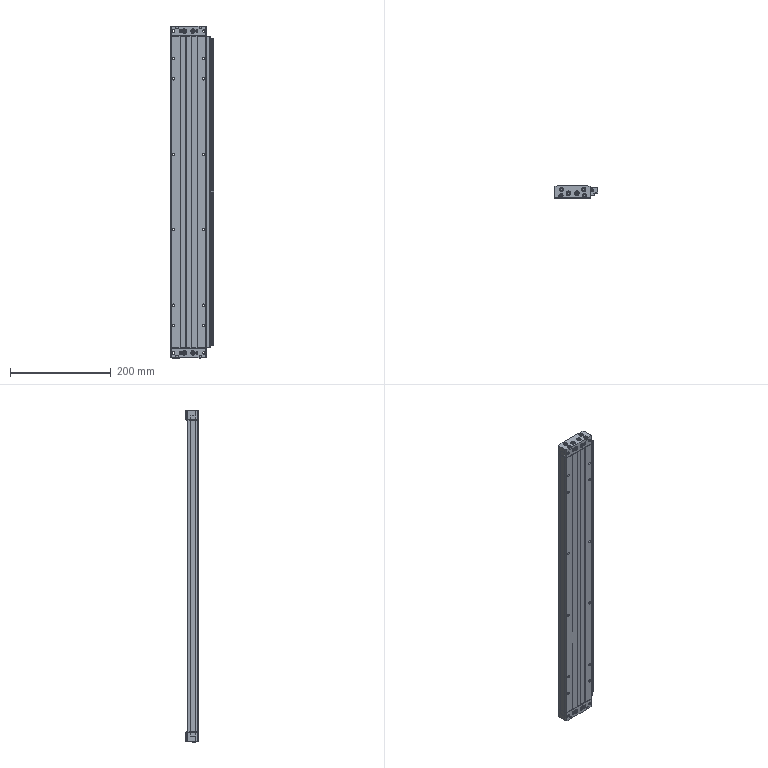Part | SolidWorks | features BaseBody 1 | 1 solid | 859 faces | box 85.5 x 24 x 660 mm | volume 981928 mm3 | cylinder 341 | plane 298 | spline 128 | cone 92 | commonest cylinder face diameters 8 x52 0.4 x48 3 x48 4.7 x32 2 x28 4.134 x20